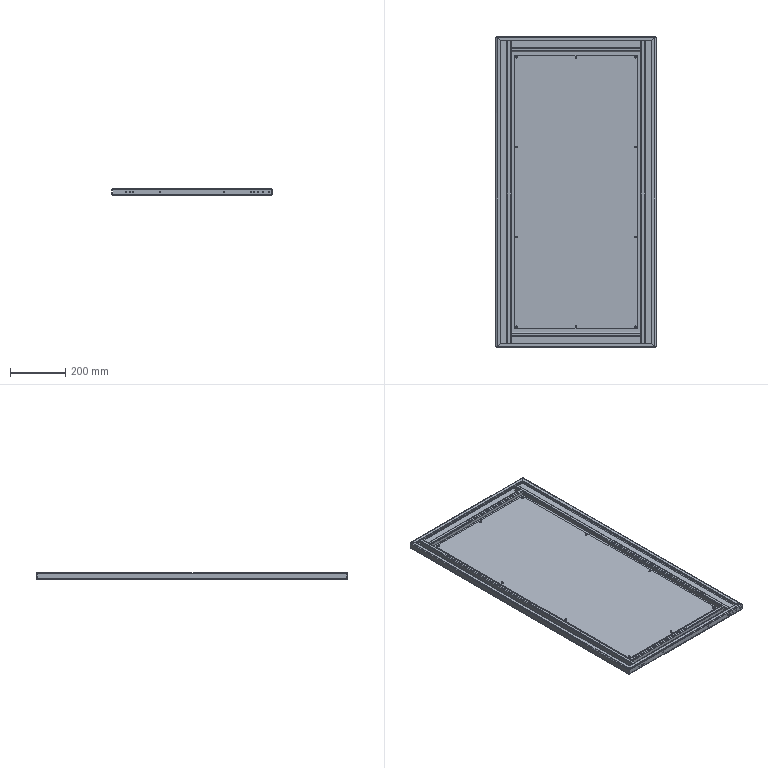Part | NX | features BREP 6 | 6 solids | 292 faces | box 580 x 1126 x 25 mm | volume 3144306 mm3 | plane 130 | cylinder 126 | cone 20 | spline 16 | commonest cylinder face diameters 4.2 x24 5 x20 5.8 x20 3.3 x16 4 x16 7 x8